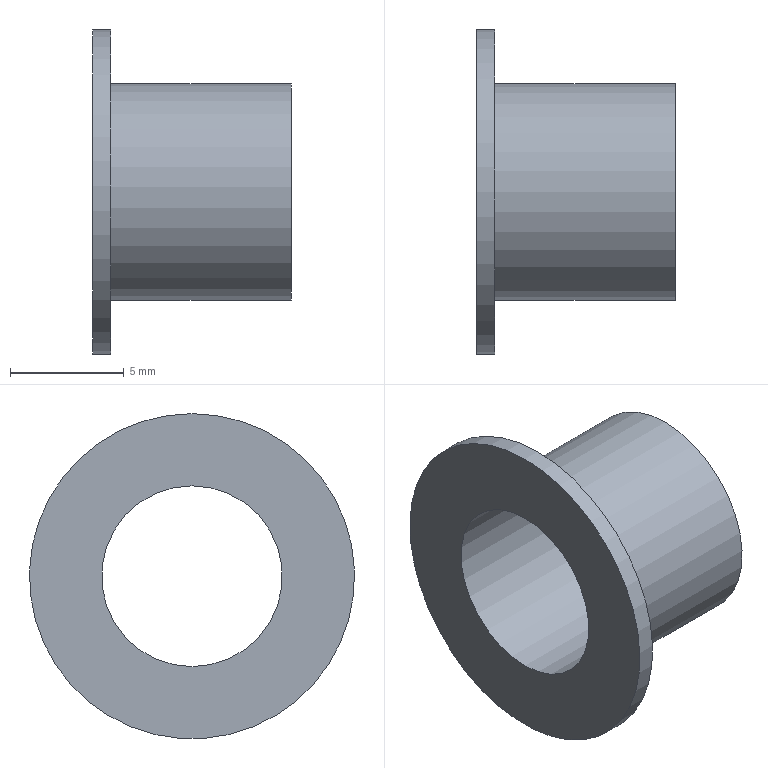Part | NX | features Igus GFI bushings(0.313 X 0.375) 2 | 1 solid | 6 faces | box 8.725 x 14.275 x 14.275 mm | volume 260.439 mm3 | plane 3 | cylinder 3 | commonest cylinder face diameters 7.938 x1 9.525 x1 14.275 x1
STEP:
#1=CARTESIAN_POINT('',(0.,0.,3.969));
#2=VERTEX_POINT('',#1);
#3=CARTESIAN_POINT('',(0.,0.,0.));
#4=DIRECTION('',(-1.,0.,0.));
#5=DIRECTION('',(0.,0.,1.));
#6=AXIS2_PLACEMENT_3D('',#3,#4,#5);
#7=CIRCLE('',#6,3.969);
#8=EDGE_CURVE('',#2,#2,#7,.T.);
#9=ORIENTED_EDGE('',*,*,#8,.F.);
#10=EDGE_LOOP('',(#9));
#11=FACE_BOUND('',#10,.T.);
#12=CARTESIAN_POINT('',(0.,0.,7.137));
#13=VERTEX_POINT('',#12);
#14=CARTESIAN_POINT('',(0.,0.,0.));
#15=DIRECTION('',(-1.,0.,0.));
#16=DIRECTION('',(0.,0.,1.));
#17=AXIS2_PLACEMENT_3D('',#14,#15,#16);
#18=CIRCLE('',#17,7.137);
#19=EDGE_CURVE('',#13,#13,#18,.T.);
#20=ORIENTED_EDGE('',*,*,#19,.T.);
#21=EDGE_LOOP('',(#20));
#22=FACE_BOUND('',#21,.T.);
#23=CARTESIAN_POINT('',(0.,3.969,0.));
#24=DIRECTION('',(1.,0.,0.));
#25=DIRECTION('',(0.,0.,-1.));
#26=AXIS2_PLACEMENT_3D('',#23,#24,#25);
#27=PLANE('',#26);
#28=ADVANCED_FACE('',(#11,#22),#27,.F.);
#29=ORIENTED_EDGE('',*,*,#19,.F.);
#30=EDGE_LOOP('',(#29));
#31=FACE_BOUND('',#30,.T.);
#32=CARTESIAN_POINT('',(0.7937,0.,7.137));
#33=VERTEX_POINT('',#32);
#34=CARTESIAN_POINT('',(0.7937,0.,0.));
#35=DIRECTION('',(-1.,0.,0.));
#36=DIRECTION('',(0.,0.,1.));
#37=AXIS2_PLACEMENT_3D('',#34,#35,#36);
#38=CIRCLE('',#37,7.137);
#39=EDGE_CURVE('',#33,#33,#38,.T.);
#40=ORIENTED_EDGE('',*,*,#39,.T.);
#41=EDGE_LOOP('',(#40));
#42=FACE_BOUND('',#41,.T.);
#43=CARTESIAN_POINT('',(0.,0.,0.));
#44=DIRECTION('',(-1.,0.,0.));
#45=DIRECTION('',(0.,0.,1.));
#46=AXIS2_PLACEMENT_3D('',#43,#44,#45);
#47=CYLINDRICAL_SURFACE('',#46,7.137);
#48=ADVANCED_FACE('',(#31,#42),#47,.T.);
#49=ORIENTED_EDGE('',*,*,#39,.F.);
#50=EDGE_LOOP('',(#49));
#51=FACE_BOUND('',#50,.T.);
#52=CARTESIAN_POINT('',(0.7937,0.,4.763));
#53=VERTEX_POINT('',#52);
#54=CARTESIAN_POINT('',(0.7937,0.,0.));
#55=DIRECTION('',(-1.,0.,0.));
#56=DIRECTION('',(0.,0.,1.));
#57=AXIS2_PLACEMENT_3D('',#54,#55,#56);
#58=CIRCLE('',#57,4.763);
#59=EDGE_CURVE('',#53,#53,#58,.T.);
#60=ORIENTED_EDGE('',*,*,#59,.T.);
#61=EDGE_LOOP('',(#60));
#62=FACE_BOUND('',#61,.T.);
#63=CARTESIAN_POINT('',(0.7937,4.763,0.));
#64=DIRECTION('',(-1.,0.,0.));
#65=DIRECTION('',(0.,0.,1.));
#66=AXIS2_PLACEMENT_3D('',#63,#64,#65);
#67=PLANE('',#66);
#68=ADVANCED_FACE('',(#51,#62),#67,.F.);
#69=ORIENTED_EDGE('',*,*,#59,.F.);
#70=EDGE_LOOP('',(#69));
#71=FACE_BOUND('',#70,.T.);
#72=CARTESIAN_POINT('',(8.725,0.,4.763));
#73=VERTEX_POINT('',#72);
#74=CARTESIAN_POINT('',(8.725,0.,0.));
#75=DIRECTION('',(-1.,0.,0.));
#76=DIRECTION('',(0.,0.,1.));
#77=AXIS2_PLACEMENT_3D('',#74,#75,#76);
#78=CIRCLE('',#77,4.763);
#79=EDGE_CURVE('',#73,#73,#78,.T.);
#80=ORIENTED_EDGE('',*,*,#79,.T.);
#81=EDGE_LOOP('',(#80));
#82=FACE_BOUND('',#81,.T.);
#83=CARTESIAN_POINT('',(0.,0.,0.));
#84=DIRECTION('',(-1.,0.,0.));
#85=DIRECTION('',(0.,0.,1.));
#86=AXIS2_PLACEMENT_3D('',#83,#84,#85);
#87=CYLINDRICAL_SURFACE('',#86,4.763);
#88=ADVANCED_FACE('',(#71,#82),#87,.T.);
#89=ORIENTED_EDGE('',*,*,#79,.F.);
#90=EDGE_LOOP('',(#89));
#91=FACE_BOUND('',#90,.T.);
#92=CARTESIAN_POINT('',(8.725,0.,3.969));
#93=VERTEX_POINT('',#92);
#94=CARTESIAN_POINT('',(8.725,0.,0.));
#95=DIRECTION('',(-1.,0.,0.));
#96=DIRECTION('',(0.,0.,1.));
#97=AXIS2_PLACEMENT_3D('',#94,#95,#96);
#98=CIRCLE('',#97,3.969);
#99=EDGE_CURVE('',#93,#93,#98,.T.);
#100=ORIENTED_EDGE('',*,*,#99,.T.);
#101=EDGE_LOOP('',(#100));
#102=FACE_BOUND('',#101,.T.);
#103=CARTESIAN_POINT('',(8.725,3.969,0.));
#104=DIRECTION('',(-1.,0.,0.));
#105=DIRECTION('',(0.,0.,1.));
#106=AXIS2_PLACEMENT_3D('',#103,#104,#105);
#107=PLANE('',#106);
#108=ADVANCED_FACE('',(#91,#102),#107,.F.);
#109=ORIENTED_EDGE('',*,*,#99,.F.);
#110=EDGE_LOOP('',(#109));
#111=FACE_BOUND('',#110,.T.);
#112=ORIENTED_EDGE('',*,*,#8,.T.);
#113=EDGE_LOOP('',(#112));
#114=FACE_BOUND('',#113,.T.);
#115=CARTESIAN_POINT('',(0.,0.,0.));
#116=DIRECTION('',(-1.,0.,0.));
#117=DIRECTION('',(0.,0.,1.));
#118=AXIS2_PLACEMENT_3D('',#115,#116,#117);
#119=CYLINDRICAL_SURFACE('',#118,3.969);
#120=ADVANCED_FACE('',(#111,#114),#119,.F.);
#121=CLOSED_SHELL('',(#28,#48,#68,#88,#108,#120));
#122=MANIFOLD_SOLID_BREP('',#121);
#123=(LENGTH_UNIT()NAMED_UNIT(*)SI_UNIT(.MILLI.,.METRE.));
#124=UNCERTAINTY_MEASURE_WITH_UNIT(LENGTH_MEASURE(0.00001),#123,'','');
#125=(NAMED_UNIT(*)PLANE_ANGLE_UNIT()SI_UNIT($,.RADIAN.));
#126=(NAMED_UNIT(*)SI_UNIT($,.STERADIAN.)SOLID_ANGLE_UNIT());
#127=(GEOMETRIC_REPRESENTATION_CONTEXT(3)GLOBAL_UNCERTAINTY_ASSIGNED_CONTEXT((#124))GLOBAL_UNIT_ASSIGNED_CONTEXT((#123,#125,#126))REPRESENTATION_CONTEXT('',''));
#128=ADVANCED_BREP_SHAPE_REPRESENTATION('',(#122),#127);